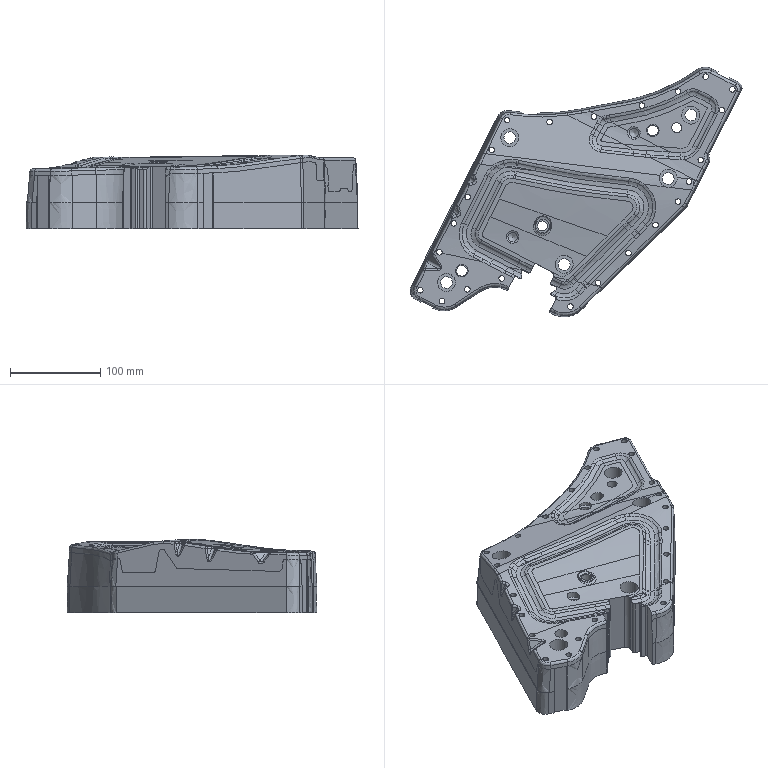Part | STEP file | gslz 2016.10.28-13_id26_x_t | 1 solid | 441 faces | box 366.996 x 275.807 x 81.669 mm | volume 3693467 mm3 | spline 229 | cylinder 109 | plane 65 | other 28 | sphere 6 | cone 4 | commonest cylinder face diameters 10.3 x25 6.2 x23 5.5 x17 0.6 x8 3 x7 13 x5